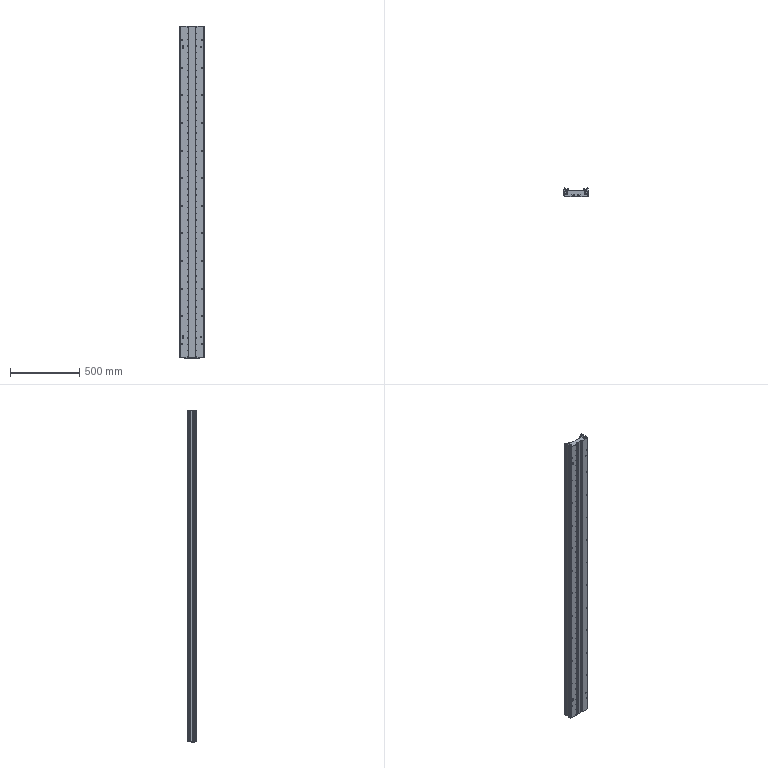Part | SolidWorks | features BaseBody 3 | 3 solids | 1096 faces | box 175 x 66 x 2404 mm | volume 15856732 mm3 | cylinder 609 | plane 271 | cone 216 | commonest cylinder face diameters 4.2 x216 0.6 x161 6.6 x96 11 x48 3.3 x33 2 x20